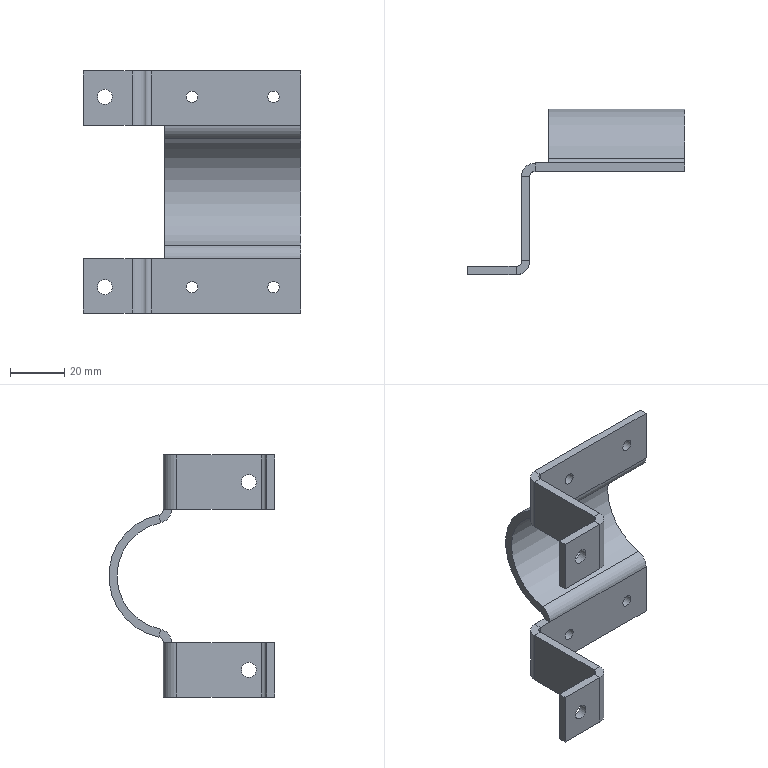Part | NX | 1 solid | 64 faces | box 80 x 61 x 88.99 mm | volume 23619 mm3 | plane 42 | cylinder 22 | commonest cylinder face diameters 4 x6 10 x6 4.2 x4 5.5 x4 40 x1 46 x1